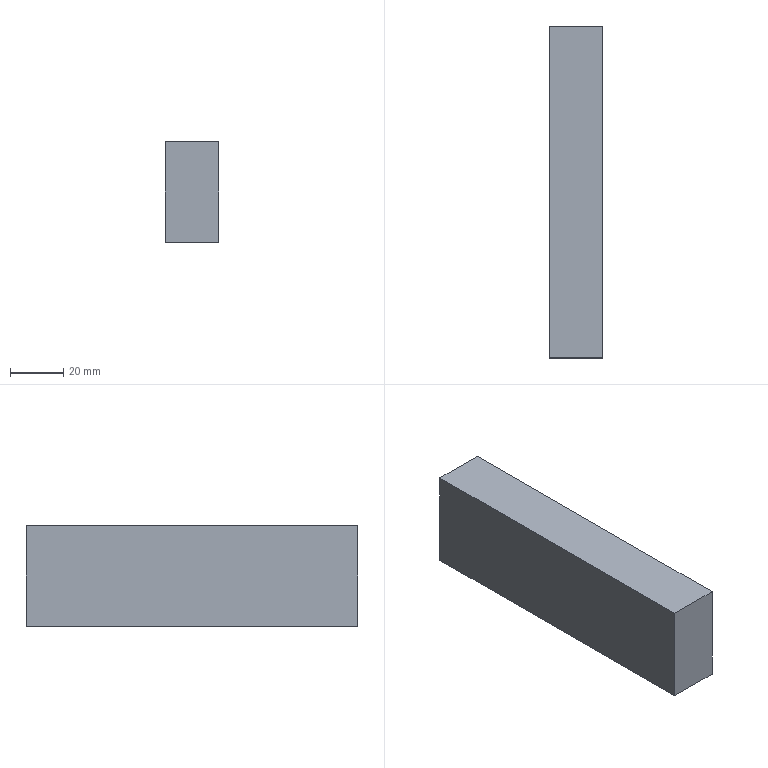Part | NX | features solid 2 | 1 solid | 6 faces | box 20 x 125 x 38 mm | volume 95000 mm3 | plane 6
STEP:
#1=CARTESIAN_POINT('',(-770.,900.,-316.));
#2=VERTEX_POINT('',#1);
#3=CARTESIAN_POINT('',(-750.,900.,-316.));
#4=VERTEX_POINT('',#3);
#5=CARTESIAN_POINT('',(-770.,900.,-316.));
#6=DIRECTION('',(1.,0.,0.));
#7=VECTOR('',#6,1000.);
#8=LINE('',#5,#7);
#9=EDGE_CURVE('',#2,#4,#8,.T.);
#10=ORIENTED_EDGE('',*,*,#9,.F.);
#11=CARTESIAN_POINT('',(-770.,900.,-354.));
#12=VERTEX_POINT('',#11);
#13=CARTESIAN_POINT('',(-770.,900.,-345.));
#14=DIRECTION('',(0.,0.,-1.));
#15=VECTOR('',#14,1000.);
#16=LINE('',#13,#15);
#17=EDGE_CURVE('',#2,#12,#16,.T.);
#18=ORIENTED_EDGE('',*,*,#17,.T.);
#19=CARTESIAN_POINT('',(-750.,900.,-354.));
#20=VERTEX_POINT('',#19);
#21=CARTESIAN_POINT('',(-770.,900.,-354.));
#22=DIRECTION('',(1.,0.,0.));
#23=VECTOR('',#22,1000.);
#24=LINE('',#21,#23);
#25=EDGE_CURVE('',#12,#20,#24,.T.);
#26=ORIENTED_EDGE('',*,*,#25,.T.);
#27=CARTESIAN_POINT('',(-750.,900.,-345.));
#28=DIRECTION('',(0.,0.,-1.));
#29=VECTOR('',#28,1000.);
#30=LINE('',#27,#29);
#31=EDGE_CURVE('',#4,#20,#30,.T.);
#32=ORIENTED_EDGE('',*,*,#31,.F.);
#33=EDGE_LOOP('',(#10,#18,#26,#32));
#34=FACE_BOUND('',#33,.T.);
#35=CARTESIAN_POINT('',(-750.,900.,-316.));
#36=DIRECTION('',(0.,-1.,0.));
#37=DIRECTION('',(0.,0.,-1.));
#38=AXIS2_PLACEMENT_3D('',#35,#36,#37);
#39=PLANE('',#38);
#40=ADVANCED_FACE('',(#34),#39,.T.);
#41=CARTESIAN_POINT('',(-750.,1025.,-354.));
#42=VERTEX_POINT('',#41);
#43=CARTESIAN_POINT('',(-750.,1025.,-316.));
#44=VERTEX_POINT('',#43);
#45=CARTESIAN_POINT('',(-750.,1025.,-345.));
#46=DIRECTION('',(0.,0.,1.));
#47=VECTOR('',#46,1000.);
#48=LINE('',#45,#47);
#49=EDGE_CURVE('',#42,#44,#48,.T.);
#50=ORIENTED_EDGE('',*,*,#49,.F.);
#51=CARTESIAN_POINT('',(-770.,1025.,-354.));
#52=VERTEX_POINT('',#51);
#53=CARTESIAN_POINT('',(-770.,1025.,-354.));
#54=DIRECTION('',(1.,0.,0.));
#55=VECTOR('',#54,1000.);
#56=LINE('',#53,#55);
#57=EDGE_CURVE('',#52,#42,#56,.T.);
#58=ORIENTED_EDGE('',*,*,#57,.F.);
#59=CARTESIAN_POINT('',(-770.,1025.,-316.));
#60=VERTEX_POINT('',#59);
#61=CARTESIAN_POINT('',(-770.,1025.,-345.));
#62=DIRECTION('',(0.,0.,1.));
#63=VECTOR('',#62,1000.);
#64=LINE('',#61,#63);
#65=EDGE_CURVE('',#52,#60,#64,.T.);
#66=ORIENTED_EDGE('',*,*,#65,.T.);
#67=CARTESIAN_POINT('',(-770.,1025.,-316.));
#68=DIRECTION('',(1.,0.,0.));
#69=VECTOR('',#68,1000.);
#70=LINE('',#67,#69);
#71=EDGE_CURVE('',#60,#44,#70,.T.);
#72=ORIENTED_EDGE('',*,*,#71,.T.);
#73=EDGE_LOOP('',(#50,#58,#66,#72));
#74=FACE_BOUND('',#73,.T.);
#75=CARTESIAN_POINT('',(-770.,1025.,-355.));
#76=DIRECTION('',(0.,1.,0.));
#77=DIRECTION('',(0.,0.,1.));
#78=AXIS2_PLACEMENT_3D('',#75,#76,#77);
#79=PLANE('',#78);
#80=ADVANCED_FACE('',(#74),#79,.T.);
#81=CARTESIAN_POINT('',(-750.,971.25,-316.));
#82=DIRECTION('',(0.,-1.,0.));
#83=VECTOR('',#82,1000.);
#84=LINE('',#81,#83);
#85=EDGE_CURVE('',#44,#4,#84,.T.);
#86=ORIENTED_EDGE('',*,*,#85,.T.);
#87=ORIENTED_EDGE('',*,*,#31,.T.);
#88=CARTESIAN_POINT('',(-750.,971.25,-354.));
#89=DIRECTION('',(0.,-1.,0.));
#90=VECTOR('',#89,1000.);
#91=LINE('',#88,#90);
#92=EDGE_CURVE('',#42,#20,#91,.T.);
#93=ORIENTED_EDGE('',*,*,#92,.F.);
#94=ORIENTED_EDGE('',*,*,#49,.T.);
#95=EDGE_LOOP('',(#86,#87,#93,#94));
#96=FACE_BOUND('',#95,.T.);
#97=CARTESIAN_POINT('',(-750.,971.25,-345.));
#98=DIRECTION('',(1.,0.,0.));
#99=DIRECTION('',(0.,0.,-1.));
#100=AXIS2_PLACEMENT_3D('',#97,#98,#99);
#101=PLANE('',#100);
#102=ADVANCED_FACE('',(#96),#101,.T.);
#103=ORIENTED_EDGE('',*,*,#17,.F.);
#104=CARTESIAN_POINT('',(-770.,971.25,-316.));
#105=DIRECTION('',(0.,-1.,0.));
#106=VECTOR('',#105,1000.);
#107=LINE('',#104,#106);
#108=EDGE_CURVE('',#60,#2,#107,.T.);
#109=ORIENTED_EDGE('',*,*,#108,.F.);
#110=ORIENTED_EDGE('',*,*,#65,.F.);
#111=CARTESIAN_POINT('',(-770.,971.25,-354.));
#112=DIRECTION('',(0.,-1.,0.));
#113=VECTOR('',#112,1000.);
#114=LINE('',#111,#113);
#115=EDGE_CURVE('',#52,#12,#114,.T.);
#116=ORIENTED_EDGE('',*,*,#115,.T.);
#117=EDGE_LOOP('',(#103,#109,#110,#116));
#118=FACE_BOUND('',#117,.T.);
#119=CARTESIAN_POINT('',(-770.,971.25,-345.));
#120=DIRECTION('',(1.,0.,0.));
#121=DIRECTION('',(0.,0.,-1.));
#122=AXIS2_PLACEMENT_3D('',#119,#120,#121);
#123=PLANE('',#122);
#124=ADVANCED_FACE('',(#118),#123,.F.);
#125=ORIENTED_EDGE('',*,*,#25,.F.);
#126=ORIENTED_EDGE('',*,*,#115,.F.);
#127=ORIENTED_EDGE('',*,*,#57,.T.);
#128=ORIENTED_EDGE('',*,*,#92,.T.);
#129=EDGE_LOOP('',(#125,#126,#127,#128));
#130=FACE_BOUND('',#129,.T.);
#131=CARTESIAN_POINT('',(-770.,1055.,-354.));
#132=DIRECTION('',(0.,0.,1.));
#133=DIRECTION('',(1.,0.,0.));
#134=AXIS2_PLACEMENT_3D('',#131,#132,#133);
#135=PLANE('',#134);
#136=ADVANCED_FACE('',(#130),#135,.F.);
#137=ORIENTED_EDGE('',*,*,#108,.T.);
#138=ORIENTED_EDGE('',*,*,#9,.T.);
#139=ORIENTED_EDGE('',*,*,#85,.F.);
#140=ORIENTED_EDGE('',*,*,#71,.F.);
#141=EDGE_LOOP('',(#137,#138,#139,#140));
#142=FACE_BOUND('',#141,.T.);
#143=CARTESIAN_POINT('',(-770.,1030.,-316.));
#144=DIRECTION('',(0.,0.,1.));
#145=DIRECTION('',(1.,0.,0.));
#146=AXIS2_PLACEMENT_3D('',#143,#144,#145);
#147=PLANE('',#146);
#148=ADVANCED_FACE('',(#142),#147,.T.);
#149=CLOSED_SHELL('',(#40,#80,#102,#124,#136,#148));
#150=MANIFOLD_SOLID_BREP('',#149);
#151=(LENGTH_UNIT()NAMED_UNIT(*)SI_UNIT(.MILLI.,.METRE.));
#152=UNCERTAINTY_MEASURE_WITH_UNIT(LENGTH_MEASURE(0.00001),#151,'','');
#153=(NAMED_UNIT(*)PLANE_ANGLE_UNIT()SI_UNIT($,.RADIAN.));
#154=(NAMED_UNIT(*)SI_UNIT($,.STERADIAN.)SOLID_ANGLE_UNIT());
#155=(GEOMETRIC_REPRESENTATION_CONTEXT(3)GLOBAL_UNCERTAINTY_ASSIGNED_CONTEXT((#152))GLOBAL_UNIT_ASSIGNED_CONTEXT((#151,#153,#154))REPRESENTATION_CONTEXT('',''));
#156=ADVANCED_BREP_SHAPE_REPRESENTATION('',(#150),#155);